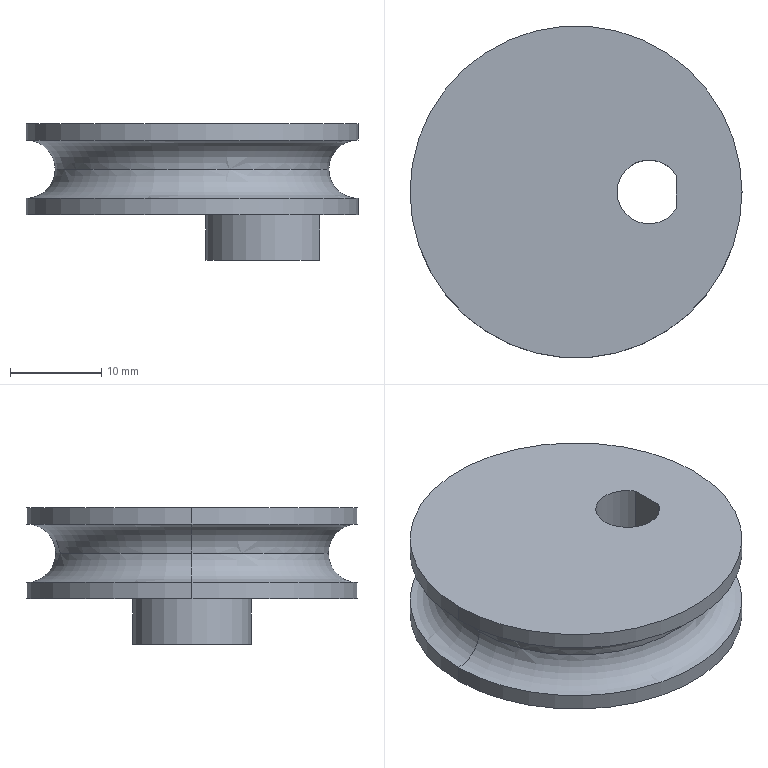Part | SolidWorks | features 3DProfileFeature 1, Extrusion 1, HoleWzd 1, ICE 1, Revolution 1 | 1 solid | 18 faces | box 36.4 x 36.4 x 15 mm | volume 8786 mm3 | cylinder 9 | plane 5 | torus 4 | commonest cylinder face diameters 36.4 x4 2.5 x2 7 x2 13 x1
STEP:
#1=CARTESIAN_POINT('',(18.2,0.,3.2));
#2=VERTEX_POINT('',#1);
#3=CARTESIAN_POINT('',(15.,0.,0.));
#4=VERTEX_POINT('',#3);
#5=CARTESIAN_POINT('',(18.2,0.,0.));
#6=DIRECTION('',(0.,-1.,0.));
#7=DIRECTION('',(0.,0.,-1.));
#8=AXIS2_PLACEMENT_3D('',#5,#6,#7);
#9=CIRCLE('',#8,3.2);
#10=EDGE_CURVE('',#2,#4,#9,.T.);
#11=ORIENTED_EDGE('',*,*,#10,.T.);
#12=CARTESIAN_POINT('',(-15.,0.,0.));
#13=VERTEX_POINT('',#12);
#14=CARTESIAN_POINT('',(0.,0.,0.));
#15=DIRECTION('',(0.,0.,1.));
#16=DIRECTION('',(1.,0.,0.));
#17=AXIS2_PLACEMENT_3D('',#14,#15,#16);
#18=CIRCLE('',#17,15.);
#19=EDGE_CURVE('',#4,#13,#18,.T.);
#20=ORIENTED_EDGE('',*,*,#19,.T.);
#21=CARTESIAN_POINT('',(-18.2,0.,3.2));
#22=VERTEX_POINT('',#21);
#23=CARTESIAN_POINT('',(-18.2,0.,0.));
#24=DIRECTION('',(0.,1.,0.));
#25=DIRECTION('',(-1.,0.,0.));
#26=AXIS2_PLACEMENT_3D('',#23,#24,#25);
#27=CIRCLE('',#26,3.2);
#28=EDGE_CURVE('',#22,#13,#27,.T.);
#29=ORIENTED_EDGE('',*,*,#28,.F.);
#30=CARTESIAN_POINT('',(0.,0.,3.2));
#31=DIRECTION('',(0.,0.,1.));
#32=DIRECTION('',(1.,0.,0.));
#33=AXIS2_PLACEMENT_3D('',#30,#31,#32);
#34=CIRCLE('',#33,18.2);
#35=EDGE_CURVE('',#2,#22,#34,.T.);
#36=ORIENTED_EDGE('',*,*,#35,.F.);
#37=EDGE_LOOP('',(#11,#20,#29,#36));
#38=FACE_OUTER_BOUND('',#37,.T.);
#39=CARTESIAN_POINT('',(0.,0.,0.));
#40=DIRECTION('',(0.,0.,1.));
#41=DIRECTION('',(1.,0.,0.));
#42=AXIS2_PLACEMENT_3D('',#39,#40,#41);
#43=TOROIDAL_SURFACE('',#42,18.2,3.2);
#44=ADVANCED_FACE('',(#38),#43,.F.);
#45=ORIENTED_EDGE('',*,*,#28,.T.);
#46=CARTESIAN_POINT('',(0.,0.,0.));
#47=DIRECTION('',(0.,0.,1.));
#48=DIRECTION('',(1.,0.,0.));
#49=AXIS2_PLACEMENT_3D('',#46,#47,#48);
#50=CIRCLE('',#49,15.);
#51=EDGE_CURVE('',#13,#4,#50,.T.);
#52=ORIENTED_EDGE('',*,*,#51,.T.);
#53=ORIENTED_EDGE('',*,*,#10,.F.);
#54=CARTESIAN_POINT('',(0.,0.,3.2));
#55=DIRECTION('',(0.,0.,1.));
#56=DIRECTION('',(1.,0.,0.));
#57=AXIS2_PLACEMENT_3D('',#54,#55,#56);
#58=CIRCLE('',#57,18.2);
#59=EDGE_CURVE('',#22,#2,#58,.T.);
#60=ORIENTED_EDGE('',*,*,#59,.F.);
#61=EDGE_LOOP('',(#45,#52,#53,#60));
#62=FACE_OUTER_BOUND('',#61,.T.);
#63=CARTESIAN_POINT('',(0.,0.,0.));
#64=DIRECTION('',(0.,0.,1.));
#65=DIRECTION('',(1.,0.,0.));
#66=AXIS2_PLACEMENT_3D('',#63,#64,#65);
#67=TOROIDAL_SURFACE('',#66,18.2,3.2);
#68=ADVANCED_FACE('',(#62),#67,.F.);
#69=CARTESIAN_POINT('',(11.,0.,-6.25));
#70=VERTEX_POINT('',#69);
#71=CARTESIAN_POINT('',(11.,0.,-8.75));
#72=VERTEX_POINT('',#71);
#73=CARTESIAN_POINT('',(11.,0.,-7.5));
#74=DIRECTION('',(1.,0.,0.));
#75=DIRECTION('',(0.,0.,-1.));
#76=AXIS2_PLACEMENT_3D('',#73,#74,#75);
#77=CIRCLE('',#76,1.25);
#78=EDGE_CURVE('',#70,#72,#77,.T.);
#79=ORIENTED_EDGE('',*,*,#78,.F.);
#80=CARTESIAN_POINT('',(14.,0.,-6.25));
#81=VERTEX_POINT('',#80);
#82=CARTESIAN_POINT('',(14.,0.,-6.25));
#83=DIRECTION('',(1.,0.,0.));
#84=VECTOR('',#83,1000.);
#85=LINE('',#82,#84);
#86=EDGE_CURVE('',#70,#81,#85,.T.);
#87=ORIENTED_EDGE('',*,*,#86,.T.);
#88=CARTESIAN_POINT('',(14.,0.,-8.75));
#89=VERTEX_POINT('',#88);
#90=CARTESIAN_POINT('',(14.,0.,-7.5));
#91=DIRECTION('',(1.,0.,0.));
#92=DIRECTION('',(0.,0.,-1.));
#93=AXIS2_PLACEMENT_3D('',#90,#91,#92);
#94=CIRCLE('',#93,1.25);
#95=EDGE_CURVE('',#81,#89,#94,.T.);
#96=ORIENTED_EDGE('',*,*,#95,.T.);
#97=CARTESIAN_POINT('',(14.,0.,-8.75));
#98=DIRECTION('',(1.,0.,0.));
#99=VECTOR('',#98,1000.);
#100=LINE('',#97,#99);
#101=EDGE_CURVE('',#72,#89,#100,.T.);
#102=ORIENTED_EDGE('',*,*,#101,.F.);
#103=EDGE_LOOP('',(#79,#87,#96,#102));
#104=FACE_OUTER_BOUND('',#103,.T.);
#105=CARTESIAN_POINT('',(14.,0.,-7.5));
#106=DIRECTION('',(1.,0.,0.));
#107=DIRECTION('',(0.,0.,-1.));
#108=AXIS2_PLACEMENT_3D('',#105,#106,#107);
#109=CYLINDRICAL_SURFACE('',#108,1.25);
#110=ADVANCED_FACE('',(#104),#109,.F.);
#111=ORIENTED_EDGE('',*,*,#35,.T.);
#112=CARTESIAN_POINT('',(-18.2,0.,5.));
#113=VERTEX_POINT('',#112);
#114=CARTESIAN_POINT('',(-18.2,0.,0.));
#115=DIRECTION('',(0.,0.,1.));
#116=VECTOR('',#115,1000.);
#117=LINE('',#114,#116);
#118=EDGE_CURVE('',#22,#113,#117,.T.);
#119=ORIENTED_EDGE('',*,*,#118,.T.);
#120=CARTESIAN_POINT('',(18.2,0.,5.));
#121=VERTEX_POINT('',#120);
#122=CARTESIAN_POINT('',(0.,0.,5.));
#123=DIRECTION('',(0.,0.,1.));
#124=DIRECTION('',(1.,0.,0.));
#125=AXIS2_PLACEMENT_3D('',#122,#123,#124);
#126=CIRCLE('',#125,18.2);
#127=EDGE_CURVE('',#121,#113,#126,.T.);
#128=ORIENTED_EDGE('',*,*,#127,.F.);
#129=CARTESIAN_POINT('',(18.2,0.,0.));
#130=DIRECTION('',(0.,0.,1.));
#131=VECTOR('',#130,1000.);
#132=LINE('',#129,#131);
#133=EDGE_CURVE('',#2,#121,#132,.T.);
#134=ORIENTED_EDGE('',*,*,#133,.F.);
#135=EDGE_LOOP('',(#111,#119,#128,#134));
#136=FACE_OUTER_BOUND('',#135,.T.);
#137=CARTESIAN_POINT('',(0.,0.,0.));
#138=DIRECTION('',(0.,0.,1.));
#139=DIRECTION('',(1.,0.,0.));
#140=AXIS2_PLACEMENT_3D('',#137,#138,#139);
#141=CYLINDRICAL_SURFACE('',#140,18.2);
#142=ADVANCED_FACE('',(#136),#141,.T.);
#143=CARTESIAN_POINT('',(18.2,0.,-5.));
#144=VERTEX_POINT('',#143);
#145=CARTESIAN_POINT('',(-18.2,0.,-5.));
#146=VERTEX_POINT('',#145);
#147=CARTESIAN_POINT('',(0.,0.,-5.));
#148=DIRECTION('',(0.,0.,1.));
#149=DIRECTION('',(1.,0.,0.));
#150=AXIS2_PLACEMENT_3D('',#147,#148,#149);
#151=CIRCLE('',#150,18.2);
#152=EDGE_CURVE('',#144,#146,#151,.T.);
#153=ORIENTED_EDGE('',*,*,#152,.T.);
#154=CARTESIAN_POINT('',(-18.2,0.,-3.2));
#155=VERTEX_POINT('',#154);
#156=CARTESIAN_POINT('',(-18.2,0.,0.));
#157=DIRECTION('',(0.,0.,1.));
#158=VECTOR('',#157,1000.);
#159=LINE('',#156,#158);
#160=EDGE_CURVE('',#146,#155,#159,.T.);
#161=ORIENTED_EDGE('',*,*,#160,.T.);
#162=CARTESIAN_POINT('',(18.2,0.,-3.2));
#163=VERTEX_POINT('',#162);
#164=CARTESIAN_POINT('',(0.,0.,-3.2));
#165=DIRECTION('',(0.,0.,1.));
#166=DIRECTION('',(1.,0.,0.));
#167=AXIS2_PLACEMENT_3D('',#164,#165,#166);
#168=CIRCLE('',#167,18.2);
#169=EDGE_CURVE('',#163,#155,#168,.T.);
#170=ORIENTED_EDGE('',*,*,#169,.F.);
#171=CARTESIAN_POINT('',(18.2,0.,0.));
#172=DIRECTION('',(0.,0.,1.));
#173=VECTOR('',#172,1000.);
#174=LINE('',#171,#173);
#175=EDGE_CURVE('',#144,#163,#174,.T.);
#176=ORIENTED_EDGE('',*,*,#175,.F.);
#177=EDGE_LOOP('',(#153,#161,#170,#176));
#178=FACE_OUTER_BOUND('',#177,.T.);
#179=CARTESIAN_POINT('',(0.,0.,0.));
#180=DIRECTION('',(0.,0.,1.));
#181=DIRECTION('',(1.,0.,0.));
#182=AXIS2_PLACEMENT_3D('',#179,#180,#181);
#183=CYLINDRICAL_SURFACE('',#182,18.2);
#184=ADVANCED_FACE('',(#178),#183,.T.);
#185=ORIENTED_EDGE('',*,*,#51,.F.);
#186=CARTESIAN_POINT('',(-18.2,0.,0.));
#187=DIRECTION('',(0.,1.,0.));
#188=DIRECTION('',(-1.,0.,0.));
#189=AXIS2_PLACEMENT_3D('',#186,#187,#188);
#190=CIRCLE('',#189,3.2);
#191=EDGE_CURVE('',#13,#155,#190,.T.);
#192=ORIENTED_EDGE('',*,*,#191,.T.);
#193=CARTESIAN_POINT('',(0.,0.,-3.2));
#194=DIRECTION('',(0.,0.,1.));
#195=DIRECTION('',(1.,0.,0.));
#196=AXIS2_PLACEMENT_3D('',#193,#194,#195);
#197=CIRCLE('',#196,18.2);
#198=EDGE_CURVE('',#155,#163,#197,.T.);
#199=ORIENTED_EDGE('',*,*,#198,.T.);
#200=CARTESIAN_POINT('',(18.2,0.,0.));
#201=DIRECTION('',(0.,-1.,0.));
#202=DIRECTION('',(0.,0.,-1.));
#203=AXIS2_PLACEMENT_3D('',#200,#201,#202);
#204=CIRCLE('',#203,3.2);
#205=EDGE_CURVE('',#4,#163,#204,.T.);
#206=ORIENTED_EDGE('',*,*,#205,.F.);
#207=EDGE_LOOP('',(#185,#192,#199,#206));
#208=FACE_OUTER_BOUND('',#207,.T.);
#209=CARTESIAN_POINT('',(0.,0.,0.));
#210=DIRECTION('',(0.,0.,1.));
#211=DIRECTION('',(1.,0.,0.));
#212=AXIS2_PLACEMENT_3D('',#209,#210,#211);
#213=TOROIDAL_SURFACE('',#212,18.2,3.2);
#214=ADVANCED_FACE('',(#208),#213,.F.);
#215=CARTESIAN_POINT('',(11.,1.803,5.));
#216=VERTEX_POINT('',#215);
#217=CARTESIAN_POINT('',(4.5,0.,5.));
#218=VERTEX_POINT('',#217);
#219=CARTESIAN_POINT('',(8.,0.,5.));
#220=DIRECTION('',(0.,0.,1.));
#221=DIRECTION('',(1.,0.,0.));
#222=AXIS2_PLACEMENT_3D('',#219,#220,#221);
#223=CIRCLE('',#222,3.5);
#224=EDGE_CURVE('',#216,#218,#223,.T.);
#225=ORIENTED_EDGE('',*,*,#224,.T.);
#226=CARTESIAN_POINT('',(4.5,0.,-10.));
#227=VERTEX_POINT('',#226);
#228=CARTESIAN_POINT('',(4.5,0.,5.));
#229=DIRECTION('',(0.,0.,-1.));
#230=VECTOR('',#229,1000.);
#231=LINE('',#228,#230);
#232=EDGE_CURVE('',#218,#227,#231,.T.);
#233=ORIENTED_EDGE('',*,*,#232,.T.);
#234=CARTESIAN_POINT('',(11.,1.803,-10.));
#235=VERTEX_POINT('',#234);
#236=CARTESIAN_POINT('',(8.,0.,-10.));
#237=DIRECTION('',(0.,0.,1.));
#238=DIRECTION('',(1.,0.,0.));
#239=AXIS2_PLACEMENT_3D('',#236,#237,#238);
#240=CIRCLE('',#239,3.5);
#241=EDGE_CURVE('',#235,#227,#240,.T.);
#242=ORIENTED_EDGE('',*,*,#241,.F.);
#243=CARTESIAN_POINT('',(11.,1.803,5.));
#244=DIRECTION('',(0.,0.,-1.));
#245=VECTOR('',#244,1000.);
#246=LINE('',#243,#245);
#247=EDGE_CURVE('',#216,#235,#246,.T.);
#248=ORIENTED_EDGE('',*,*,#247,.F.);
#249=EDGE_LOOP('',(#225,#233,#242,#248));
#250=FACE_OUTER_BOUND('',#249,.T.);
#251=CARTESIAN_POINT('',(8.,0.,5.));
#252=DIRECTION('',(0.,0.,-1.));
#253=DIRECTION('',(-1.,0.,0.));
#254=AXIS2_PLACEMENT_3D('',#251,#252,#253);
#255=CYLINDRICAL_SURFACE('',#254,3.5);
#256=ADVANCED_FACE('',(#250),#255,.F.);
#257=ORIENTED_EDGE('',*,*,#232,.F.);
#258=CARTESIAN_POINT('',(11.,-1.803,5.));
#259=VERTEX_POINT('',#258);
#260=CARTESIAN_POINT('',(8.,0.,5.));
#261=DIRECTION('',(0.,0.,1.));
#262=DIRECTION('',(1.,0.,0.));
#263=AXIS2_PLACEMENT_3D('',#260,#261,#262);
#264=CIRCLE('',#263,3.5);
#265=EDGE_CURVE('',#218,#259,#264,.T.);
#266=ORIENTED_EDGE('',*,*,#265,.T.);
#267=CARTESIAN_POINT('',(11.,-1.803,-10.));
#268=VERTEX_POINT('',#267);
#269=CARTESIAN_POINT('',(11.,-1.803,5.));
#270=DIRECTION('',(0.,0.,-1.));
#271=VECTOR('',#270,1000.);
#272=LINE('',#269,#271);
#273=EDGE_CURVE('',#259,#268,#272,.T.);
#274=ORIENTED_EDGE('',*,*,#273,.T.);
#275=CARTESIAN_POINT('',(8.,0.,-10.));
#276=DIRECTION('',(0.,0.,1.));
#277=DIRECTION('',(1.,0.,0.));
#278=AXIS2_PLACEMENT_3D('',#275,#276,#277);
#279=CIRCLE('',#278,3.5);
#280=EDGE_CURVE('',#227,#268,#279,.T.);
#281=ORIENTED_EDGE('',*,*,#280,.F.);
#282=EDGE_LOOP('',(#257,#266,#274,#281));
#283=FACE_OUTER_BOUND('',#282,.T.);
#284=CARTESIAN_POINT('',(8.,0.,5.));
#285=DIRECTION('',(0.,0.,-1.));
#286=DIRECTION('',(-1.,0.,0.));
#287=AXIS2_PLACEMENT_3D('',#284,#285,#286);
#288=CYLINDRICAL_SURFACE('',#287,3.5);
#289=ADVANCED_FACE('',(#283),#288,.F.);
#290=CARTESIAN_POINT('',(11.,0.,-7.5));
#291=DIRECTION('',(1.,0.,0.));
#292=DIRECTION('',(0.,0.,-1.));
#293=AXIS2_PLACEMENT_3D('',#290,#291,#292);
#294=CIRCLE('',#293,1.25);
#295=EDGE_CURVE('',#72,#70,#294,.T.);
#296=ORIENTED_EDGE('',*,*,#295,.T.);
#297=ORIENTED_EDGE('',*,*,#78,.T.);
#298=EDGE_LOOP('',(#296,#297));
#299=FACE_BOUND('',#298,.T.);
#300=ORIENTED_EDGE('',*,*,#247,.T.);
#301=CARTESIAN_POINT('',(11.,-1.803,-10.));
#302=DIRECTION('',(0.,1.,0.));
#303=VECTOR('',#302,1000.);
#304=LINE('',#301,#303);
#305=EDGE_CURVE('',#268,#235,#304,.T.);
#306=ORIENTED_EDGE('',*,*,#305,.F.);
#307=ORIENTED_EDGE('',*,*,#273,.F.);
#308=CARTESIAN_POINT('',(11.,0.,5.));
#309=DIRECTION('',(0.,-1.,0.));
#310=VECTOR('',#309,1000.);
#311=LINE('',#308,#310);
#312=EDGE_CURVE('',#216,#259,#311,.T.);
#313=ORIENTED_EDGE('',*,*,#312,.F.);
#314=EDGE_LOOP('',(#300,#306,#307,#313));
#315=FACE_OUTER_BOUND('',#314,.T.);
#316=CARTESIAN_POINT('',(11.,0.,5.));
#317=DIRECTION('',(1.,0.,0.));
#318=DIRECTION('',(0.,0.,-1.));
#319=AXIS2_PLACEMENT_3D('',#316,#317,#318);
#320=PLANE('',#319);
#321=ADVANCED_FACE('',(#299,#315),#320,.F.);
#322=ORIENTED_EDGE('',*,*,#224,.F.);
#323=ORIENTED_EDGE('',*,*,#312,.T.);
#324=ORIENTED_EDGE('',*,*,#265,.F.);
#325=EDGE_LOOP('',(#322,#323,#324));
#326=FACE_BOUND('',#325,.T.);
#327=ORIENTED_EDGE('',*,*,#127,.T.);
#328=CARTESIAN_POINT('',(0.,0.,5.));
#329=DIRECTION('',(0.,0.,1.));
#330=DIRECTION('',(1.,0.,0.));
#331=AXIS2_PLACEMENT_3D('',#328,#329,#330);
#332=CIRCLE('',#331,18.2);
#333=EDGE_CURVE('',#113,#121,#332,.T.);
#334=ORIENTED_EDGE('',*,*,#333,.T.);
#335=EDGE_LOOP('',(#327,#334));
#336=FACE_OUTER_BOUND('',#335,.T.);
#337=CARTESIAN_POINT('',(0.,0.,5.));
#338=DIRECTION('',(0.,0.,1.));
#339=DIRECTION('',(1.,0.,0.));
#340=AXIS2_PLACEMENT_3D('',#337,#338,#339);
#341=PLANE('',#340);
#342=ADVANCED_FACE('',(#326,#336),#341,.T.);
#343=CARTESIAN_POINT('',(14.,-2.5,-5.));
#344=VERTEX_POINT('',#343);
#345=CARTESIAN_POINT('',(14.,2.5,-5.));
#346=VERTEX_POINT('',#345);
#347=CARTESIAN_POINT('',(14.,-2.5,-5.));
#348=DIRECTION('',(0.,1.,0.));
#349=VECTOR('',#348,1000.);
#350=LINE('',#347,#349);
#351=EDGE_CURVE('',#344,#346,#350,.T.);
#352=ORIENTED_EDGE('',*,*,#351,.T.);
#353=CARTESIAN_POINT('',(8.,0.,-5.));
#354=DIRECTION('',(0.,0.,1.));
#355=DIRECTION('',(1.,0.,0.));
#356=AXIS2_PLACEMENT_3D('',#353,#354,#355);
#357=CIRCLE('',#356,6.5);
#358=EDGE_CURVE('',#346,#344,#357,.T.);
#359=ORIENTED_EDGE('',*,*,#358,.T.);
#360=EDGE_LOOP('',(#352,#359));
#361=FACE_BOUND('',#360,.T.);
#362=ORIENTED_EDGE('',*,*,#152,.F.);
#363=CARTESIAN_POINT('',(0.,0.,-5.));
#364=DIRECTION('',(0.,0.,1.));
#365=DIRECTION('',(1.,0.,0.));
#366=AXIS2_PLACEMENT_3D('',#363,#364,#365);
#367=CIRCLE('',#366,18.2);
#368=EDGE_CURVE('',#146,#144,#367,.T.);
#369=ORIENTED_EDGE('',*,*,#368,.F.);
#370=EDGE_LOOP('',(#362,#369));
#371=FACE_OUTER_BOUND('',#370,.T.);
#372=CARTESIAN_POINT('',(0.,0.,-5.));
#373=DIRECTION('',(0.,0.,1.));
#374=DIRECTION('',(1.,0.,0.));
#375=AXIS2_PLACEMENT_3D('',#372,#373,#374);
#376=PLANE('',#375);
#377=ADVANCED_FACE('',(#361,#371),#376,.F.);
#378=ORIENTED_EDGE('',*,*,#19,.F.);
#379=ORIENTED_EDGE('',*,*,#205,.T.);
#380=ORIENTED_EDGE('',*,*,#169,.T.);
#381=ORIENTED_EDGE('',*,*,#191,.F.);
#382=EDGE_LOOP('',(#378,#379,#380,#381));
#383=FACE_OUTER_BOUND('',#382,.T.);
#384=CARTESIAN_POINT('',(0.,0.,0.));
#385=DIRECTION('',(0.,0.,1.));
#386=DIRECTION('',(1.,0.,0.));
#387=AXIS2_PLACEMENT_3D('',#384,#385,#386);
#388=TOROIDAL_SURFACE('',#387,18.2,3.2);
#389=ADVANCED_FACE('',(#383),#388,.F.);
#390=ORIENTED_EDGE('',*,*,#160,.F.);
#391=ORIENTED_EDGE('',*,*,#368,.T.);
#392=ORIENTED_EDGE('',*,*,#175,.T.);
#393=ORIENTED_EDGE('',*,*,#198,.F.);
#394=EDGE_LOOP('',(#390,#391,#392,#393));
#395=FACE_OUTER_BOUND('',#394,.T.);
#396=CARTESIAN_POINT('',(0.,0.,0.));
#397=DIRECTION('',(0.,0.,1.));
#398=DIRECTION('',(1.,0.,0.));
#399=AXIS2_PLACEMENT_3D('',#396,#397,#398);
#400=CYLINDRICAL_SURFACE('',#399,18.2);
#401=ADVANCED_FACE('',(#395),#400,.T.);
#402=ORIENTED_EDGE('',*,*,#118,.F.);
#403=ORIENTED_EDGE('',*,*,#59,.T.);
#404=ORIENTED_EDGE('',*,*,#133,.T.);
#405=ORIENTED_EDGE('',*,*,#333,.F.);
#406=EDGE_LOOP('',(#402,#403,#404,#405));
#407=FACE_OUTER_BOUND('',#406,.T.);
#408=CARTESIAN_POINT('',(0.,0.,0.));
#409=DIRECTION('',(0.,0.,1.));
#410=DIRECTION('',(1.,0.,0.));
#411=AXIS2_PLACEMENT_3D('',#408,#409,#410);
#412=CYLINDRICAL_SURFACE('',#411,18.2);
#413=ADVANCED_FACE('',(#407),#412,.T.);
#414=ORIENTED_EDGE('',*,*,#358,.F.);
#415=CARTESIAN_POINT('',(14.,2.5,-10.));
#416=VERTEX_POINT('',#415);
#417=CARTESIAN_POINT('',(14.,2.5,-10.));
#418=DIRECTION('',(0.,0.,1.));
#419=VECTOR('',#418,1000.);
#420=LINE('',#417,#419);
#421=EDGE_CURVE('',#416,#346,#420,.T.);
#422=ORIENTED_EDGE('',*,*,#421,.F.);
#423=CARTESIAN_POINT('',(14.,-2.5,-10.));
#424=VERTEX_POINT('',#423);
#425=CARTESIAN_POINT('',(8.,0.,-10.));
#426=DIRECTION('',(0.,0.,1.));
#427=DIRECTION('',(1.,0.,0.));
#428=AXIS2_PLACEMENT_3D('',#425,#426,#427);
#429=CIRCLE('',#428,6.5);
#430=EDGE_CURVE('',#416,#424,#429,.T.);
#431=ORIENTED_EDGE('',*,*,#430,.T.);
#432=CARTESIAN_POINT('',(14.,-2.5,-10.));
#433=DIRECTION('',(0.,0.,1.));
#434=VECTOR('',#433,1000.);
#435=LINE('',#432,#434);
#436=EDGE_CURVE('',#424,#344,#435,.T.);
#437=ORIENTED_EDGE('',*,*,#436,.T.);
#438=EDGE_LOOP('',(#414,#422,#431,#437));
#439=FACE_OUTER_BOUND('',#438,.T.);
#440=CARTESIAN_POINT('',(8.,0.,-10.));
#441=DIRECTION('',(0.,0.,1.));
#442=DIRECTION('',(1.,0.,0.));
#443=AXIS2_PLACEMENT_3D('',#440,#441,#442);
#444=CYLINDRICAL_SURFACE('',#443,6.5);
#445=ADVANCED_FACE('',(#439),#444,.T.);
#446=CARTESIAN_POINT('',(14.,0.,-7.5));
#447=DIRECTION('',(1.,0.,0.));
#448=DIRECTION('',(0.,0.,-1.));
#449=AXIS2_PLACEMENT_3D('',#446,#447,#448);
#450=CIRCLE('',#449,1.25);
#451=EDGE_CURVE('',#89,#81,#450,.T.);
#452=ORIENTED_EDGE('',*,*,#451,.F.);
#453=ORIENTED_EDGE('',*,*,#95,.F.);
#454=EDGE_LOOP('',(#452,#453));
#455=FACE_BOUND('',#454,.T.);
#456=ORIENTED_EDGE('',*,*,#351,.F.);
#457=ORIENTED_EDGE('',*,*,#436,.F.);
#458=CARTESIAN_POINT('',(14.,-2.5,-10.));
#459=DIRECTION('',(0.,1.,0.));
#460=VECTOR('',#459,1000.);
#461=LINE('',#458,#460);
#462=EDGE_CURVE('',#424,#416,#461,.T.);
#463=ORIENTED_EDGE('',*,*,#462,.T.);
#464=ORIENTED_EDGE('',*,*,#421,.T.);
#465=EDGE_LOOP('',(#456,#457,#463,#464));
#466=FACE_OUTER_BOUND('',#465,.T.);
#467=CARTESIAN_POINT('',(14.,-2.5,-10.));
#468=DIRECTION('',(1.,0.,0.));
#469=DIRECTION('',(0.,0.,-1.));
#470=AXIS2_PLACEMENT_3D('',#467,#468,#469);
#471=PLANE('',#470);
#472=ADVANCED_FACE('',(#455,#466),#471,.T.);
#473=ORIENTED_EDGE('',*,*,#305,.T.);
#474=ORIENTED_EDGE('',*,*,#241,.T.);
#475=ORIENTED_EDGE('',*,*,#280,.T.);
#476=EDGE_LOOP('',(#473,#474,#475));
#477=FACE_BOUND('',#476,.T.);
#478=ORIENTED_EDGE('',*,*,#430,.F.);
#479=ORIENTED_EDGE('',*,*,#462,.F.);
#480=EDGE_LOOP('',(#478,#479));
#481=FACE_OUTER_BOUND('',#480,.T.);
#482=CARTESIAN_POINT('',(8.,0.,-10.));
#483=DIRECTION('',(0.,0.,1.));
#484=DIRECTION('',(1.,0.,0.));
#485=AXIS2_PLACEMENT_3D('',#482,#483,#484);
#486=PLANE('',#485);
#487=ADVANCED_FACE('',(#477,#481),#486,.F.);
#488=ORIENTED_EDGE('',*,*,#86,.F.);
#489=ORIENTED_EDGE('',*,*,#295,.F.);
#490=ORIENTED_EDGE('',*,*,#101,.T.);
#491=ORIENTED_EDGE('',*,*,#451,.T.);
#492=EDGE_LOOP('',(#488,#489,#490,#491));
#493=FACE_OUTER_BOUND('',#492,.T.);
#494=CARTESIAN_POINT('',(14.,0.,-7.5));
#495=DIRECTION('',(1.,0.,0.));
#496=DIRECTION('',(0.,0.,-1.));
#497=AXIS2_PLACEMENT_3D('',#494,#495,#496);
#498=CYLINDRICAL_SURFACE('',#497,1.25);
#499=ADVANCED_FACE('',(#493),#498,.F.);
#500=CLOSED_SHELL('',(#44,#68,#110,#142,#184,#214,#256,#289,#321,#342,#377,#389,#401,#413,#445,#472,#487,#499));
#501=MANIFOLD_SOLID_BREP('',#500);
#502=CARTESIAN_POINT('',(0.,0.,0.));
#503=DIRECTION('',(0.,0.,1.));
#504=DIRECTION('',(1.,0.,0.));
#505=AXIS2_PLACEMENT_3D('',#502,#503,#504);
#506=(LENGTH_UNIT()NAMED_UNIT(*)SI_UNIT(.MILLI.,.METRE.));
#507=UNCERTAINTY_MEASURE_WITH_UNIT(LENGTH_MEASURE(0.00001),#506,'','');
#508=(NAMED_UNIT(*)PLANE_ANGLE_UNIT()SI_UNIT($,.RADIAN.));
#509=(NAMED_UNIT(*)SI_UNIT($,.STERADIAN.)SOLID_ANGLE_UNIT());
#510=(GEOMETRIC_REPRESENTATION_CONTEXT(3)GLOBAL_UNCERTAINTY_ASSIGNED_CONTEXT((#507))GLOBAL_UNIT_ASSIGNED_CONTEXT((#506,#508,#509))REPRESENTATION_CONTEXT('',''));
#511=ADVANCED_BREP_SHAPE_REPRESENTATION('',(#501,#505),#510);